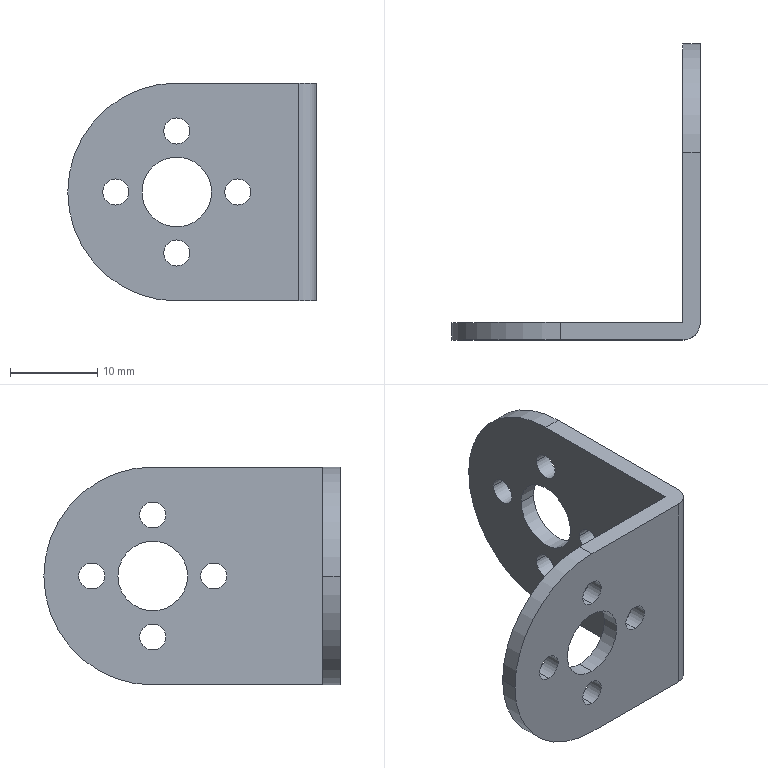Part | SolidWorks | features Fillet 3, ICE 3, Extrusion 1 | 1 solid | 31 faces | box 28.5 x 34 x 25 mm | volume 2421 mm3 | cylinder 25 | plane 6 | commonest cylinder face diameters 3 x16 8 x4 25 x4 4 x1
STEP:
#1=CARTESIAN_POINT('',(-8.75,-15.,14.));
#2=VERTEX_POINT('',#1);
#3=CARTESIAN_POINT('',(-8.75,-15.,11.));
#4=VERTEX_POINT('',#3);
#5=CARTESIAN_POINT('',(-8.75,-15.,12.5));
#6=DIRECTION('',(0.,-1.,0.));
#7=DIRECTION('',(1.,0.,0.));
#8=AXIS2_PLACEMENT_3D('',#5,#6,#7);
#9=CIRCLE('',#8,1.5);
#10=EDGE_CURVE('',#2,#4,#9,.T.);
#11=ORIENTED_EDGE('',*,*,#10,.F.);
#12=CARTESIAN_POINT('',(-8.75,-17.,14.));
#13=VERTEX_POINT('',#12);
#14=CARTESIAN_POINT('',(-8.75,17.,14.));
#15=DIRECTION('',(0.,-1.,0.));
#16=VECTOR('',#15,1000.);
#17=LINE('',#14,#16);
#18=EDGE_CURVE('',#2,#13,#17,.T.);
#19=ORIENTED_EDGE('',*,*,#18,.T.);
#20=CARTESIAN_POINT('',(-8.75,-17.,11.));
#21=VERTEX_POINT('',#20);
#22=CARTESIAN_POINT('',(-8.75,-17.,12.5));
#23=DIRECTION('',(0.,-1.,0.));
#24=DIRECTION('',(0.,0.,-1.));
#25=AXIS2_PLACEMENT_3D('',#22,#23,#24);
#26=CIRCLE('',#25,1.5);
#27=EDGE_CURVE('',#13,#21,#26,.T.);
#28=ORIENTED_EDGE('',*,*,#27,.T.);
#29=CARTESIAN_POINT('',(-8.75,17.,11.));
#30=DIRECTION('',(0.,-1.,0.));
#31=VECTOR('',#30,1000.);
#32=LINE('',#29,#31);
#33=EDGE_CURVE('',#4,#21,#32,.T.);
#34=ORIENTED_EDGE('',*,*,#33,.F.);
#35=EDGE_LOOP('',(#11,#19,#28,#34));
#36=FACE_OUTER_BOUND('',#35,.T.);
#37=CARTESIAN_POINT('',(-8.75,17.,12.5));
#38=DIRECTION('',(0.,-1.,0.));
#39=DIRECTION('',(0.,0.,-1.));
#40=AXIS2_PLACEMENT_3D('',#37,#38,#39);
#41=CYLINDRICAL_SURFACE('',#40,1.5);
#42=ADVANCED_FACE('',(#36),#41,.F.);
#43=CARTESIAN_POINT('',(-1.75,-15.,21.));
#44=VERTEX_POINT('',#43);
#45=CARTESIAN_POINT('',(-1.75,-15.,18.));
#46=VERTEX_POINT('',#45);
#47=CARTESIAN_POINT('',(-1.75,-15.,19.5));
#48=DIRECTION('',(0.,-1.,0.));
#49=DIRECTION('',(1.,0.,0.));
#50=AXIS2_PLACEMENT_3D('',#47,#48,#49);
#51=CIRCLE('',#50,1.5);
#52=EDGE_CURVE('',#44,#46,#51,.T.);
#53=ORIENTED_EDGE('',*,*,#52,.F.);
#54=CARTESIAN_POINT('',(-1.75,-17.,21.));
#55=VERTEX_POINT('',#54);
#56=CARTESIAN_POINT('',(-1.75,17.,21.));
#57=DIRECTION('',(0.,-1.,0.));
#58=VECTOR('',#57,1000.);
#59=LINE('',#56,#58);
#60=EDGE_CURVE('',#44,#55,#59,.T.);
#61=ORIENTED_EDGE('',*,*,#60,.T.);
#62=CARTESIAN_POINT('',(-1.75,-17.,18.));
#63=VERTEX_POINT('',#62);
#64=CARTESIAN_POINT('',(-1.75,-17.,19.5));
#65=DIRECTION('',(0.,-1.,0.));
#66=DIRECTION('',(0.,0.,-1.));
#67=AXIS2_PLACEMENT_3D('',#64,#65,#66);
#68=CIRCLE('',#67,1.5);
#69=EDGE_CURVE('',#55,#63,#68,.T.);
#70=ORIENTED_EDGE('',*,*,#69,.T.);
#71=CARTESIAN_POINT('',(-1.75,17.,18.));
#72=DIRECTION('',(0.,-1.,0.));
#73=VECTOR('',#72,1000.);
#74=LINE('',#71,#73);
#75=EDGE_CURVE('',#46,#63,#74,.T.);
#76=ORIENTED_EDGE('',*,*,#75,.F.);
#77=EDGE_LOOP('',(#53,#61,#70,#76));
#78=FACE_OUTER_BOUND('',#77,.T.);
#79=CARTESIAN_POINT('',(-1.75,17.,19.5));
#80=DIRECTION('',(0.,-1.,0.));
#81=DIRECTION('',(0.,0.,-1.));
#82=AXIS2_PLACEMENT_3D('',#79,#80,#81);
#83=CYLINDRICAL_SURFACE('',#82,1.5);
#84=ADVANCED_FACE('',(#78),#83,.F.);
#85=CARTESIAN_POINT('',(5.25,-15.,14.));
#86=VERTEX_POINT('',#85);
#87=CARTESIAN_POINT('',(5.25,-15.,11.));
#88=VERTEX_POINT('',#87);
#89=CARTESIAN_POINT('',(5.25,-15.,12.5));
#90=DIRECTION('',(0.,-1.,0.));
#91=DIRECTION('',(1.,0.,0.));
#92=AXIS2_PLACEMENT_3D('',#89,#90,#91);
#93=CIRCLE('',#92,1.5);
#94=EDGE_CURVE('',#86,#88,#93,.T.);
#95=ORIENTED_EDGE('',*,*,#94,.F.);
#96=CARTESIAN_POINT('',(5.25,-17.,14.));
#97=VERTEX_POINT('',#96);
#98=CARTESIAN_POINT('',(5.25,17.,14.));
#99=DIRECTION('',(0.,-1.,0.));
#100=VECTOR('',#99,1000.);
#101=LINE('',#98,#100);
#102=EDGE_CURVE('',#86,#97,#101,.T.);
#103=ORIENTED_EDGE('',*,*,#102,.T.);
#104=CARTESIAN_POINT('',(5.25,-17.,11.));
#105=VERTEX_POINT('',#104);
#106=CARTESIAN_POINT('',(5.25,-17.,12.5));
#107=DIRECTION('',(0.,-1.,0.));
#108=DIRECTION('',(0.,0.,-1.));
#109=AXIS2_PLACEMENT_3D('',#106,#107,#108);
#110=CIRCLE('',#109,1.5);
#111=EDGE_CURVE('',#97,#105,#110,.T.);
#112=ORIENTED_EDGE('',*,*,#111,.T.);
#113=CARTESIAN_POINT('',(5.25,17.,11.));
#114=DIRECTION('',(0.,-1.,0.));
#115=VECTOR('',#114,1000.);
#116=LINE('',#113,#115);
#117=EDGE_CURVE('',#88,#105,#116,.T.);
#118=ORIENTED_EDGE('',*,*,#117,.F.);
#119=EDGE_LOOP('',(#95,#103,#112,#118));
#120=FACE_OUTER_BOUND('',#119,.T.);
#121=CARTESIAN_POINT('',(5.25,17.,12.5));
#122=DIRECTION('',(0.,-1.,0.));
#123=DIRECTION('',(0.,0.,-1.));
#124=AXIS2_PLACEMENT_3D('',#121,#122,#123);
#125=CYLINDRICAL_SURFACE('',#124,1.5);
#126=ADVANCED_FACE('',(#120),#125,.F.);
#127=CARTESIAN_POINT('',(-1.75,-15.,7.));
#128=VERTEX_POINT('',#127);
#129=CARTESIAN_POINT('',(-1.75,-15.,4.));
#130=VERTEX_POINT('',#129);
#131=CARTESIAN_POINT('',(-1.75,-15.,5.5));
#132=DIRECTION('',(0.,-1.,0.));
#133=DIRECTION('',(1.,0.,0.));
#134=AXIS2_PLACEMENT_3D('',#131,#132,#133);
#135=CIRCLE('',#134,1.5);
#136=EDGE_CURVE('',#128,#130,#135,.T.);
#137=ORIENTED_EDGE('',*,*,#136,.F.);
#138=CARTESIAN_POINT('',(-1.75,-17.,7.));
#139=VERTEX_POINT('',#138);
#140=CARTESIAN_POINT('',(-1.75,17.,7.));
#141=DIRECTION('',(0.,-1.,0.));
#142=VECTOR('',#141,1000.);
#143=LINE('',#140,#142);
#144=EDGE_CURVE('',#128,#139,#143,.T.);
#145=ORIENTED_EDGE('',*,*,#144,.T.);
#146=CARTESIAN_POINT('',(-1.75,-17.,4.));
#147=VERTEX_POINT('',#146);
#148=CARTESIAN_POINT('',(-1.75,-17.,5.5));
#149=DIRECTION('',(0.,-1.,0.));
#150=DIRECTION('',(0.,0.,-1.));
#151=AXIS2_PLACEMENT_3D('',#148,#149,#150);
#152=CIRCLE('',#151,1.5);
#153=EDGE_CURVE('',#139,#147,#152,.T.);
#154=ORIENTED_EDGE('',*,*,#153,.T.);
#155=CARTESIAN_POINT('',(-1.75,17.,4.));
#156=DIRECTION('',(0.,-1.,0.));
#157=VECTOR('',#156,1000.);
#158=LINE('',#155,#157);
#159=EDGE_CURVE('',#130,#147,#158,.T.);
#160=ORIENTED_EDGE('',*,*,#159,.F.);
#161=EDGE_LOOP('',(#137,#145,#154,#160));
#162=FACE_OUTER_BOUND('',#161,.T.);
#163=CARTESIAN_POINT('',(-1.75,17.,5.5));
#164=DIRECTION('',(0.,-1.,0.));
#165=DIRECTION('',(0.,0.,-1.));
#166=AXIS2_PLACEMENT_3D('',#163,#164,#165);
#167=CYLINDRICAL_SURFACE('',#166,1.5);
#168=ADVANCED_FACE('',(#162),#167,.F.);
#169=CARTESIAN_POINT('',(-1.75,-15.,16.5));
#170=VERTEX_POINT('',#169);
#171=CARTESIAN_POINT('',(-1.75,-15.,8.5));
#172=VERTEX_POINT('',#171);
#173=CARTESIAN_POINT('',(-1.75,-15.,12.5));
#174=DIRECTION('',(0.,-1.,0.));
#175=DIRECTION('',(1.,0.,0.));
#176=AXIS2_PLACEMENT_3D('',#173,#174,#175);
#177=CIRCLE('',#176,4.);
#178=EDGE_CURVE('',#170,#172,#177,.T.);
#179=ORIENTED_EDGE('',*,*,#178,.F.);
#180=CARTESIAN_POINT('',(-1.75,-17.,16.5));
#181=VERTEX_POINT('',#180);
#182=CARTESIAN_POINT('',(-1.75,17.,16.5));
#183=DIRECTION('',(0.,-1.,0.));
#184=VECTOR('',#183,1000.);
#185=LINE('',#182,#184);
#186=EDGE_CURVE('',#170,#181,#185,.T.);
#187=ORIENTED_EDGE('',*,*,#186,.T.);
#188=CARTESIAN_POINT('',(-1.75,-17.,8.5));
#189=VERTEX_POINT('',#188);
#190=CARTESIAN_POINT('',(-1.75,-17.,12.5));
#191=DIRECTION('',(0.,-1.,0.));
#192=DIRECTION('',(0.,0.,-1.));
#193=AXIS2_PLACEMENT_3D('',#190,#191,#192);
#194=CIRCLE('',#193,4.);
#195=EDGE_CURVE('',#181,#189,#194,.T.);
#196=ORIENTED_EDGE('',*,*,#195,.T.);
#197=CARTESIAN_POINT('',(-1.75,17.,8.5));
#198=DIRECTION('',(0.,-1.,0.));
#199=VECTOR('',#198,1000.);
#200=LINE('',#197,#199);
#201=EDGE_CURVE('',#172,#189,#200,.T.);
#202=ORIENTED_EDGE('',*,*,#201,.F.);
#203=EDGE_LOOP('',(#179,#187,#196,#202));
#204=FACE_OUTER_BOUND('',#203,.T.);
#205=CARTESIAN_POINT('',(-1.75,17.,12.5));
#206=DIRECTION('',(0.,-1.,0.));
#207=DIRECTION('',(0.,0.,-1.));
#208=AXIS2_PLACEMENT_3D('',#205,#206,#207);
#209=CYLINDRICAL_SURFACE('',#208,4.);
#210=ADVANCED_FACE('',(#204),#209,.F.);
#211=CARTESIAN_POINT('',(14.25,6.,5.5));
#212=VERTEX_POINT('',#211);
#213=CARTESIAN_POINT('',(14.25,3.,5.5));
#214=VERTEX_POINT('',#213);
#215=CARTESIAN_POINT('',(14.25,4.5,5.5));
#216=DIRECTION('',(-1.,0.,0.));
#217=DIRECTION('',(0.,-1.,0.));
#218=AXIS2_PLACEMENT_3D('',#215,#216,#217);
#219=CIRCLE('',#218,1.5);
#220=EDGE_CURVE('',#212,#214,#219,.T.);
#221=ORIENTED_EDGE('',*,*,#220,.F.);
#222=CARTESIAN_POINT('',(12.25,6.,5.5));
#223=VERTEX_POINT('',#222);
#224=CARTESIAN_POINT('',(14.25,6.,5.5));
#225=DIRECTION('',(-1.,0.,0.));
#226=VECTOR('',#225,1000.);
#227=LINE('',#224,#226);
#228=EDGE_CURVE('',#212,#223,#227,.T.);
#229=ORIENTED_EDGE('',*,*,#228,.T.);
#230=CARTESIAN_POINT('',(12.25,3.,5.5));
#231=VERTEX_POINT('',#230);
#232=CARTESIAN_POINT('',(12.25,4.5,5.5));
#233=DIRECTION('',(-1.,0.,0.));
#234=DIRECTION('',(0.,-1.,0.));
#235=AXIS2_PLACEMENT_3D('',#232,#233,#234);
#236=CIRCLE('',#235,1.5);
#237=EDGE_CURVE('',#223,#231,#236,.T.);
#238=ORIENTED_EDGE('',*,*,#237,.T.);
#239=CARTESIAN_POINT('',(14.25,3.,5.5));
#240=DIRECTION('',(-1.,0.,0.));
#241=VECTOR('',#240,1000.);
#242=LINE('',#239,#241);
#243=EDGE_CURVE('',#214,#231,#242,.T.);
#244=ORIENTED_EDGE('',*,*,#243,.F.);
#245=EDGE_LOOP('',(#221,#229,#238,#244));
#246=FACE_OUTER_BOUND('',#245,.T.);
#247=CARTESIAN_POINT('',(14.25,4.5,5.5));
#248=DIRECTION('',(-1.,0.,0.));
#249=DIRECTION('',(0.,-1.,0.));
#250=AXIS2_PLACEMENT_3D('',#247,#248,#249);
#251=CYLINDRICAL_SURFACE('',#250,1.5);
#252=ADVANCED_FACE('',(#246),#251,.F.);
#253=CARTESIAN_POINT('',(14.25,13.,12.5));
#254=VERTEX_POINT('',#253);
#255=CARTESIAN_POINT('',(14.25,10.,12.5));
#256=VERTEX_POINT('',#255);
#257=CARTESIAN_POINT('',(14.25,11.5,12.5));
#258=DIRECTION('',(-1.,0.,0.));
#259=DIRECTION('',(0.,-1.,0.));
#260=AXIS2_PLACEMENT_3D('',#257,#258,#259);
#261=CIRCLE('',#260,1.5);
#262=EDGE_CURVE('',#254,#256,#261,.T.);
#263=ORIENTED_EDGE('',*,*,#262,.F.);
#264=CARTESIAN_POINT('',(12.25,13.,12.5));
#265=VERTEX_POINT('',#264);
#266=CARTESIAN_POINT('',(14.25,13.,12.5));
#267=DIRECTION('',(-1.,0.,0.));
#268=VECTOR('',#267,1000.);
#269=LINE('',#266,#268);
#270=EDGE_CURVE('',#254,#265,#269,.T.);
#271=ORIENTED_EDGE('',*,*,#270,.T.);
#272=CARTESIAN_POINT('',(12.25,10.,12.5));
#273=VERTEX_POINT('',#272);
#274=CARTESIAN_POINT('',(12.25,11.5,12.5));
#275=DIRECTION('',(-1.,0.,0.));
#276=DIRECTION('',(0.,-1.,0.));
#277=AXIS2_PLACEMENT_3D('',#274,#275,#276);
#278=CIRCLE('',#277,1.5);
#279=EDGE_CURVE('',#265,#273,#278,.T.);
#280=ORIENTED_EDGE('',*,*,#279,.T.);
#281=CARTESIAN_POINT('',(14.25,10.,12.5));
#282=DIRECTION('',(-1.,0.,0.));
#283=VECTOR('',#282,1000.);
#284=LINE('',#281,#283);
#285=EDGE_CURVE('',#256,#273,#284,.T.);
#286=ORIENTED_EDGE('',*,*,#285,.F.);
#287=EDGE_LOOP('',(#263,#271,#280,#286));
#288=FACE_OUTER_BOUND('',#287,.T.);
#289=CARTESIAN_POINT('',(14.25,11.5,12.5));
#290=DIRECTION('',(-1.,0.,0.));
#291=DIRECTION('',(0.,-1.,0.));
#292=AXIS2_PLACEMENT_3D('',#289,#290,#291);
#293=CYLINDRICAL_SURFACE('',#292,1.5);
#294=ADVANCED_FACE('',(#288),#293,.F.);
#295=CARTESIAN_POINT('',(14.25,6.,19.5));
#296=VERTEX_POINT('',#295);
#297=CARTESIAN_POINT('',(14.25,3.,19.5));
#298=VERTEX_POINT('',#297);
#299=CARTESIAN_POINT('',(14.25,4.5,19.5));
#300=DIRECTION('',(-1.,0.,0.));
#301=DIRECTION('',(0.,-1.,0.));
#302=AXIS2_PLACEMENT_3D('',#299,#300,#301);
#303=CIRCLE('',#302,1.5);
#304=EDGE_CURVE('',#296,#298,#303,.T.);
#305=ORIENTED_EDGE('',*,*,#304,.F.);
#306=CARTESIAN_POINT('',(12.25,6.,19.5));
#307=VERTEX_POINT('',#306);
#308=CARTESIAN_POINT('',(14.25,6.,19.5));
#309=DIRECTION('',(-1.,0.,0.));
#310=VECTOR('',#309,1000.);
#311=LINE('',#308,#310);
#312=EDGE_CURVE('',#296,#307,#311,.T.);
#313=ORIENTED_EDGE('',*,*,#312,.T.);
#314=CARTESIAN_POINT('',(12.25,3.,19.5));
#315=VERTEX_POINT('',#314);
#316=CARTESIAN_POINT('',(12.25,4.5,19.5));
#317=DIRECTION('',(-1.,0.,0.));
#318=DIRECTION('',(0.,-1.,0.));
#319=AXIS2_PLACEMENT_3D('',#316,#317,#318);
#320=CIRCLE('',#319,1.5);
#321=EDGE_CURVE('',#307,#315,#320,.T.);
#322=ORIENTED_EDGE('',*,*,#321,.T.);
#323=CARTESIAN_POINT('',(14.25,3.,19.5));
#324=DIRECTION('',(-1.,0.,0.));
#325=VECTOR('',#324,1000.);
#326=LINE('',#323,#325);
#327=EDGE_CURVE('',#298,#315,#326,.T.);
#328=ORIENTED_EDGE('',*,*,#327,.F.);
#329=EDGE_LOOP('',(#305,#313,#322,#328));
#330=FACE_OUTER_BOUND('',#329,.T.);
#331=CARTESIAN_POINT('',(14.25,4.5,19.5));
#332=DIRECTION('',(-1.,0.,0.));
#333=DIRECTION('',(0.,-1.,0.));
#334=AXIS2_PLACEMENT_3D('',#331,#332,#333);
#335=CYLINDRICAL_SURFACE('',#334,1.5);
#336=ADVANCED_FACE('',(#330),#335,.F.);
#337=CARTESIAN_POINT('',(14.25,-1.,12.5));
#338=VERTEX_POINT('',#337);
#339=CARTESIAN_POINT('',(14.25,-4.,12.5));
#340=VERTEX_POINT('',#339);
#341=CARTESIAN_POINT('',(14.25,-2.5,12.5));
#342=DIRECTION('',(-1.,0.,0.));
#343=DIRECTION('',(0.,-1.,0.));
#344=AXIS2_PLACEMENT_3D('',#341,#342,#343);
#345=CIRCLE('',#344,1.5);
#346=EDGE_CURVE('',#338,#340,#345,.T.);
#347=ORIENTED_EDGE('',*,*,#346,.F.);
#348=CARTESIAN_POINT('',(12.25,-1.,12.5));
#349=VERTEX_POINT('',#348);
#350=CARTESIAN_POINT('',(14.25,-1.,12.5));
#351=DIRECTION('',(-1.,0.,0.));
#352=VECTOR('',#351,1000.);
#353=LINE('',#350,#352);
#354=EDGE_CURVE('',#338,#349,#353,.T.);
#355=ORIENTED_EDGE('',*,*,#354,.T.);
#356=CARTESIAN_POINT('',(12.25,-4.,12.5));
#357=VERTEX_POINT('',#356);
#358=CARTESIAN_POINT('',(12.25,-2.5,12.5));
#359=DIRECTION('',(-1.,0.,0.));
#360=DIRECTION('',(0.,-1.,0.));
#361=AXIS2_PLACEMENT_3D('',#358,#359,#360);
#362=CIRCLE('',#361,1.5);
#363=EDGE_CURVE('',#349,#357,#362,.T.);
#364=ORIENTED_EDGE('',*,*,#363,.T.);
#365=CARTESIAN_POINT('',(14.25,-4.,12.5));
#366=DIRECTION('',(-1.,0.,0.));
#367=VECTOR('',#366,1000.);
#368=LINE('',#365,#367);
#369=EDGE_CURVE('',#340,#357,#368,.T.);
#370=ORIENTED_EDGE('',*,*,#369,.F.);
#371=EDGE_LOOP('',(#347,#355,#364,#370));
#372=FACE_OUTER_BOUND('',#371,.T.);
#373=CARTESIAN_POINT('',(14.25,-2.5,12.5));
#374=DIRECTION('',(-1.,0.,0.));
#375=DIRECTION('',(0.,-1.,0.));
#376=AXIS2_PLACEMENT_3D('',#373,#374,#375);
#377=CYLINDRICAL_SURFACE('',#376,1.5);
#378=ADVANCED_FACE('',(#372),#377,.F.);
#379=CARTESIAN_POINT('',(14.25,8.5,12.5));
#380=VERTEX_POINT('',#379);
#381=CARTESIAN_POINT('',(14.25,0.5,12.5));
#382=VERTEX_POINT('',#381);
#383=CARTESIAN_POINT('',(14.25,4.5,12.5));
#384=DIRECTION('',(-1.,0.,0.));
#385=DIRECTION('',(0.,-1.,0.));
#386=AXIS2_PLACEMENT_3D('',#383,#384,#385);
#387=CIRCLE('',#386,4.);
#388=EDGE_CURVE('',#380,#382,#387,.T.);
#389=ORIENTED_EDGE('',*,*,#388,.F.);
#390=CARTESIAN_POINT('',(12.25,8.5,12.5));
#391=VERTEX_POINT('',#390);
#392=CARTESIAN_POINT('',(14.25,8.5,12.5));
#393=DIRECTION('',(-1.,0.,0.));
#394=VECTOR('',#393,1000.);
#395=LINE('',#392,#394);
#396=EDGE_CURVE('',#380,#391,#395,.T.);
#397=ORIENTED_EDGE('',*,*,#396,.T.);
#398=CARTESIAN_POINT('',(12.25,0.5,12.5));
#399=VERTEX_POINT('',#398);
#400=CARTESIAN_POINT('',(12.25,4.5,12.5));
#401=DIRECTION('',(-1.,0.,0.));
#402=DIRECTION('',(0.,-1.,0.));
#403=AXIS2_PLACEMENT_3D('',#400,#401,#402);
#404=CIRCLE('',#403,4.);
#405=EDGE_CURVE('',#391,#399,#404,.T.);
#406=ORIENTED_EDGE('',*,*,#405,.T.);
#407=CARTESIAN_POINT('',(14.25,0.5,12.5));
#408=DIRECTION('',(-1.,0.,0.));
#409=VECTOR('',#408,1000.);
#410=LINE('',#407,#409);
#411=EDGE_CURVE('',#382,#399,#410,.T.);
#412=ORIENTED_EDGE('',*,*,#411,.F.);
#413=EDGE_LOOP('',(#389,#397,#406,#412));
#414=FACE_OUTER_BOUND('',#413,.T.);
#415=CARTESIAN_POINT('',(14.25,4.5,12.5));
#416=DIRECTION('',(-1.,0.,0.));
#417=DIRECTION('',(0.,-1.,0.));
#418=AXIS2_PLACEMENT_3D('',#415,#416,#417);
#419=CYLINDRICAL_SURFACE('',#418,4.);
#420=ADVANCED_FACE('',(#414),#419,.F.);
#421=CARTESIAN_POINT('',(14.25,4.5,5.5));
#422=DIRECTION('',(-1.,0.,0.));
#423=DIRECTION('',(0.,-1.,0.));
#424=AXIS2_PLACEMENT_3D('',#421,#422,#423);
#425=CIRCLE('',#424,1.5);
#426=EDGE_CURVE('',#214,#212,#425,.T.);
#427=ORIENTED_EDGE('',*,*,#426,.T.);
#428=ORIENTED_EDGE('',*,*,#220,.T.);
#429=EDGE_LOOP('',(#427,#428));
#430=FACE_BOUND('',#429,.T.);
#431=CARTESIAN_POINT('',(14.25,11.5,12.5));
#432=DIRECTION('',(-1.,0.,0.));
#433=DIRECTION('',(0.,-1.,0.));
#434=AXIS2_PLACEMENT_3D('',#431,#432,#433);
#435=CIRCLE('',#434,1.5);
#436=EDGE_CURVE('',#256,#254,#435,.T.);
#437=ORIENTED_EDGE('',*,*,#436,.T.);
#438=ORIENTED_EDGE('',*,*,#262,.T.);
#439=EDGE_LOOP('',(#437,#438));
#440=FACE_BOUND('',#439,.T.);
#441=CARTESIAN_POINT('',(14.25,4.5,19.5));
#442=DIRECTION('',(-1.,0.,0.));
#443=DIRECTION('',(0.,-1.,0.));
#444=AXIS2_PLACEMENT_3D('',#441,#442,#443);
#445=CIRCLE('',#444,1.5);
#446=EDGE_CURVE('',#298,#296,#445,.T.);
#447=ORIENTED_EDGE('',*,*,#446,.T.);
#448=ORIENTED_EDGE('',*,*,#304,.T.);
#449=EDGE_LOOP('',(#447,#448));
#450=FACE_BOUND('',#449,.T.);
#451=CARTESIAN_POINT('',(14.25,-2.5,12.5));
#452=DIRECTION('',(-1.,0.,0.));
#453=DIRECTION('',(0.,-1.,0.));
#454=AXIS2_PLACEMENT_3D('',#451,#452,#453);
#455=CIRCLE('',#454,1.5);
#456=EDGE_CURVE('',#340,#338,#455,.T.);
#457=ORIENTED_EDGE('',*,*,#456,.T.);
#458=ORIENTED_EDGE('',*,*,#346,.T.);
#459=EDGE_LOOP('',(#457,#458));
#460=FACE_BOUND('',#459,.T.);
#461=CARTESIAN_POINT('',(14.25,4.5,12.5));
#462=DIRECTION('',(-1.,0.,0.));
#463=DIRECTION('',(0.,-1.,0.));
#464=AXIS2_PLACEMENT_3D('',#461,#462,#463);
#465=CIRCLE('',#464,4.);
#466=EDGE_CURVE('',#382,#380,#465,.T.);
#467=ORIENTED_EDGE('',*,*,#466,.T.);
#468=ORIENTED_EDGE('',*,*,#388,.T.);
#469=EDGE_LOOP('',(#467,#468));
#470=FACE_BOUND('',#469,.T.);
#471=CARTESIAN_POINT('',(14.25,-15.,25.));
#472=VERTEX_POINT('',#471);
#473=CARTESIAN_POINT('',(14.25,4.5,25.));
#474=VERTEX_POINT('',#473);
#475=CARTESIAN_POINT('',(14.25,17.,25.));
#476=DIRECTION('',(0.,1.,0.));
#477=VECTOR('',#476,1000.);
#478=LINE('',#475,#477);
#479=EDGE_CURVE('',#472,#474,#478,.T.);
#480=ORIENTED_EDGE('',*,*,#479,.F.);
#481=CARTESIAN_POINT('',(14.25,-15.,0.));
#482=VERTEX_POINT('',#481);
#483=CARTESIAN_POINT('',(14.25,-15.,25.));
#484=DIRECTION('',(0.,0.,-1.));
#485=VECTOR('',#484,1000.);
#486=LINE('',#483,#485);
#487=EDGE_CURVE('',#472,#482,#486,.T.);
#488=ORIENTED_EDGE('',*,*,#487,.T.);
#489=CARTESIAN_POINT('',(14.25,4.5,0.));
#490=VERTEX_POINT('',#489);
#491=CARTESIAN_POINT('',(14.25,17.,0.));
#492=DIRECTION('',(0.,1.,0.));
#493=VECTOR('',#492,1000.);
#494=LINE('',#491,#493);
#495=EDGE_CURVE('',#482,#490,#494,.T.);
#496=ORIENTED_EDGE('',*,*,#495,.T.);
#497=CARTESIAN_POINT('',(14.25,17.,12.5));
#498=VERTEX_POINT('',#497);
#499=CARTESIAN_POINT('',(14.25,4.5,12.5));
#500=DIRECTION('',(1.,0.,0.));
#501=DIRECTION('',(0.,-1.,0.));
#502=AXIS2_PLACEMENT_3D('',#499,#500,#501);
#503=CIRCLE('',#502,12.5);
#504=EDGE_CURVE('',#490,#498,#503,.T.);
#505=ORIENTED_EDGE('',*,*,#504,.T.);
#506=CARTESIAN_POINT('',(14.25,4.5,12.5));
#507=DIRECTION('',(1.,0.,0.));
#508=DIRECTION('',(0.,-1.,0.));
#509=AXIS2_PLACEMENT_3D('',#506,#507,#508);
#510=CIRCLE('',#509,12.5);
#511=EDGE_CURVE('',#498,#474,#510,.T.);
#512=ORIENTED_EDGE('',*,*,#511,.T.);
#513=EDGE_LOOP('',(#480,#488,#496,#505,#512));
#514=FACE_OUTER_BOUND('',#513,.T.);
#515=CARTESIAN_POINT('',(14.25,17.,25.));
#516=DIRECTION('',(-1.,0.,0.));
#517=DIRECTION('',(0.,-1.,0.));
#518=AXIS2_PLACEMENT_3D('',#515,#516,#517);
#519=PLANE('',#518);
#520=ADVANCED_FACE('',(#430,#440,#450,#460,#470,#514),#519,.F.);
#521=CARTESIAN_POINT('',(-8.75,-17.,12.5));
#522=DIRECTION('',(0.,-1.,0.));
#523=DIRECTION('',(0.,0.,-1.));
#524=AXIS2_PLACEMENT_3D('',#521,#522,#523);
#525=CIRCLE('',#524,1.5);
#526=EDGE_CURVE('',#21,#13,#525,.T.);
#527=ORIENTED_EDGE('',*,*,#526,.F.);
#528=ORIENTED_EDGE('',*,*,#27,.F.);
#529=EDGE_LOOP('',(#527,#528));
#530=FACE_BOUND('',#529,.T.);
#531=CARTESIAN_POINT('',(-1.75,-17.,19.5));
#532=DIRECTION('',(0.,-1.,0.));
#533=DIRECTION('',(0.,0.,-1.));
#534=AXIS2_PLACEMENT_3D('',#531,#532,#533);
#535=CIRCLE('',#534,1.5);
#536=EDGE_CURVE('',#63,#55,#535,.T.);
#537=ORIENTED_EDGE('',*,*,#536,.F.);
#538=ORIENTED_EDGE('',*,*,#69,.F.);
#539=EDGE_LOOP('',(#537,#538));
#540=FACE_BOUND('',#539,.T.);
#541=CARTESIAN_POINT('',(5.25,-17.,12.5));
#542=DIRECTION('',(0.,-1.,0.));
#543=DIRECTION('',(0.,0.,-1.));
#544=AXIS2_PLACEMENT_3D('',#541,#542,#543);
#545=CIRCLE('',#544,1.5);
#546=EDGE_CURVE('',#105,#97,#545,.T.);
#547=ORIENTED_EDGE('',*,*,#546,.F.);
#548=ORIENTED_EDGE('',*,*,#111,.F.);
#549=EDGE_LOOP('',(#547,#548));
#550=FACE_BOUND('',#549,.T.);
#551=CARTESIAN_POINT('',(-1.75,-17.,5.5));
#552=DIRECTION('',(0.,-1.,0.));
#553=DIRECTION('',(0.,0.,-1.));
#554=AXIS2_PLACEMENT_3D('',#551,#552,#553);
#555=CIRCLE('',#554,1.5);
#556=EDGE_CURVE('',#147,#139,#555,.T.);
#557=ORIENTED_EDGE('',*,*,#556,.F.);
#558=ORIENTED_EDGE('',*,*,#153,.F.);
#559=EDGE_LOOP('',(#557,#558));
#560=FACE_BOUND('',#559,.T.);
#561=CARTESIAN_POINT('',(-1.75,-17.,12.5));
#562=DIRECTION('',(0.,-1.,0.));
#563=DIRECTION('',(0.,0.,-1.));
#564=AXIS2_PLACEMENT_3D('',#561,#562,#563);
#565=CIRCLE('',#564,4.);
#566=EDGE_CURVE('',#189,#181,#565,.T.);
#567=ORIENTED_EDGE('',*,*,#566,.F.);
#568=ORIENTED_EDGE('',*,*,#195,.F.);
#569=EDGE_LOOP('',(#567,#568));
#570=FACE_BOUND('',#569,.T.);
#571=CARTESIAN_POINT('',(-1.75,-17.,0.));
#572=VERTEX_POINT('',#571);
#573=CARTESIAN_POINT('',(12.25,-17.,0.));
#574=VERTEX_POINT('',#573);
#575=CARTESIAN_POINT('',(-14.25,-17.,0.));
#576=DIRECTION('',(1.,0.,0.));
#577=VECTOR('',#576,1000.);
#578=LINE('',#575,#577);
#579=EDGE_CURVE('',#572,#574,#578,.T.);
#580=ORIENTED_EDGE('',*,*,#579,.T.);
#581=CARTESIAN_POINT('',(12.25,-17.,25.));
#582=VERTEX_POINT('',#581);
#583=CARTESIAN_POINT('',(12.25,-17.,25.));
#584=DIRECTION('',(0.,0.,1.));
#585=VECTOR('',#584,1000.);
#586=LINE('',#583,#585);
#587=EDGE_CURVE('',#574,#582,#586,.T.);
#588=ORIENTED_EDGE('',*,*,#587,.T.);
#589=CARTESIAN_POINT('',(-1.75,-17.,25.));
#590=VERTEX_POINT('',#589);
#591=CARTESIAN_POINT('',(-14.25,-17.,25.));
#592=DIRECTION('',(1.,0.,0.));
#593=VECTOR('',#592,1000.);
#594=LINE('',#591,#593);
#595=EDGE_CURVE('',#590,#582,#594,.T.);
#596=ORIENTED_EDGE('',*,*,#595,.F.);
#597=CARTESIAN_POINT('',(-14.25,-17.,12.5));
#598=VERTEX_POINT('',#597);
#599=CARTESIAN_POINT('',(-1.75,-17.,12.5));
#600=DIRECTION('',(0.,-1.,0.));
#601=DIRECTION('',(0.,0.,1.));
#602=AXIS2_PLACEMENT_3D('',#599,#600,#601);
#603=CIRCLE('',#602,12.5);
#604=EDGE_CURVE('',#590,#598,#603,.T.);
#605=ORIENTED_EDGE('',*,*,#604,.T.);
#606=CARTESIAN_POINT('',(-1.75,-17.,12.5));
#607=DIRECTION('',(0.,-1.,0.));
#608=DIRECTION('',(0.,0.,1.));
#609=AXIS2_PLACEMENT_3D('',#606,#607,#608);
#610=CIRCLE('',#609,12.5);
#611=EDGE_CURVE('',#598,#572,#610,.T.);
#612=ORIENTED_EDGE('',*,*,#611,.T.);
#613=EDGE_LOOP('',(#580,#588,#596,#605,#612));
#614=FACE_OUTER_BOUND('',#613,.T.);
#615=CARTESIAN_POINT('',(-14.25,-17.,25.));
#616=DIRECTION('',(0.,1.,0.));
#617=DIRECTION('',(0.,0.,1.));
#618=AXIS2_PLACEMENT_3D('',#615,#616,#617);
#619=PLANE('',#618);
#620=ADVANCED_FACE('',(#530,#540,#550,#560,#570,#614),#619,.F.);
#621=ORIENTED_EDGE('',*,*,#595,.T.);
#622=CARTESIAN_POINT('',(12.25,-15.,25.));
#623=DIRECTION('',(0.,0.,1.));
#624=DIRECTION('',(1.,0.,0.));
#625=AXIS2_PLACEMENT_3D('',#622,#623,#624);
#626=CIRCLE('',#625,2.);
#627=EDGE_CURVE('',#582,#472,#626,.T.);
#628=ORIENTED_EDGE('',*,*,#627,.T.);
#629=ORIENTED_EDGE('',*,*,#479,.T.);
#630=CARTESIAN_POINT('',(12.25,4.5,25.));
#631=VERTEX_POINT('',#630);
#632=CARTESIAN_POINT('',(12.25,4.5,25.));
#633=DIRECTION('',(-1.,0.,0.));
#634=VECTOR('',#633,1000.);
#635=LINE('',#632,#634);
#636=EDGE_CURVE('',#474,#631,#635,.T.);
#637=ORIENTED_EDGE('',*,*,#636,.T.);
#638=CARTESIAN_POINT('',(12.25,-15.,25.));
#639=VERTEX_POINT('',#638);
#640=CARTESIAN_POINT('',(12.25,17.,25.));
#641=DIRECTION('',(0.,-1.,0.));
#642=VECTOR('',#641,1000.);
#643=LINE('',#640,#642);
#644=EDGE_CURVE('',#631,#639,#643,.T.);
#645=ORIENTED_EDGE('',*,*,#644,.T.);
#646=CARTESIAN_POINT('',(-1.75,-15.,25.));
#647=VERTEX_POINT('',#646);
#648=CARTESIAN_POINT('',(12.25,-15.,25.));
#649=DIRECTION('',(-1.,0.,0.));
#650=VECTOR('',#649,1000.);
#651=LINE('',#648,#650);
#652=EDGE_CURVE('',#639,#647,#651,.T.);
#653=ORIENTED_EDGE('',*,*,#652,.T.);
#654=CARTESIAN_POINT('',(-1.75,-17.,25.));
#655=DIRECTION('',(0.,-1.,0.));
#656=VECTOR('',#655,1000.);
#657=LINE('',#654,#656);
#658=EDGE_CURVE('',#647,#590,#657,.T.);
#659=ORIENTED_EDGE('',*,*,#658,.T.);
#660=EDGE_LOOP('',(#621,#628,#629,#637,#645,#653,#659));
#661=FACE_OUTER_BOUND('',#660,.T.);
#662=CARTESIAN_POINT('',(0.,0.,25.));
#663=DIRECTION('',(0.,0.,1.));
#664=DIRECTION('',(1.,0.,0.));
#665=AXIS2_PLACEMENT_3D('',#662,#663,#664);
#666=PLANE('',#665);
#667=ADVANCED_FACE('',(#661),#666,.T.);
#668=ORIENTED_EDGE('',*,*,#495,.F.);
#669=CARTESIAN_POINT('',(12.25,-15.,0.));
#670=DIRECTION('',(0.,0.,-1.));
#671=DIRECTION('',(1.,0.,0.));
#672=AXIS2_PLACEMENT_3D('',#669,#670,#671);
#673=CIRCLE('',#672,2.);
#674=EDGE_CURVE('',#482,#574,#673,.T.);
#675=ORIENTED_EDGE('',*,*,#674,.T.);
#676=ORIENTED_EDGE('',*,*,#579,.F.);
#677=CARTESIAN_POINT('',(-1.75,-15.,0.));
#678=VERTEX_POINT('',#677);
#679=CARTESIAN_POINT('',(-1.75,0.,0.));
#680=DIRECTION('',(0.,1.,0.));
#681=VECTOR('',#680,1000.);
#682=LINE('',#679,#681);
#683=EDGE_CURVE('',#572,#678,#682,.T.);
#684=ORIENTED_EDGE('',*,*,#683,.T.);
#685=CARTESIAN_POINT('',(12.25,-15.,0.));
#686=VERTEX_POINT('',#685);
#687=CARTESIAN_POINT('',(12.25,-15.,0.));
#688=DIRECTION('',(-1.,0.,0.));
#689=VECTOR('',#688,1000.);
#690=LINE('',#687,#689);
#691=EDGE_CURVE('',#686,#678,#690,.T.);
#692=ORIENTED_EDGE('',*,*,#691,.F.);
#693=CARTESIAN_POINT('',(12.25,4.5,0.));
#694=VERTEX_POINT('',#693);
#695=CARTESIAN_POINT('',(12.25,17.,0.));
#696=DIRECTION('',(0.,-1.,0.));
#697=VECTOR('',#696,1000.);
#698=LINE('',#695,#697);
#699=EDGE_CURVE('',#694,#686,#698,.T.);
#700=ORIENTED_EDGE('',*,*,#699,.F.);
#701=CARTESIAN_POINT('',(0.,4.5,0.));
#702=DIRECTION('',(1.,0.,0.));
#703=VECTOR('',#702,1000.);
#704=LINE('',#701,#703);
#705=EDGE_CURVE('',#694,#490,#704,.T.);
#706=ORIENTED_EDGE('',*,*,#705,.T.);
#707=EDGE_LOOP('',(#668,#675,#676,#684,#692,#700,#706));
#708=FACE_OUTER_BOUND('',#707,.T.);
#709=CARTESIAN_POINT('',(0.,0.,0.));
#710=DIRECTION('',(0.,0.,1.));
#711=DIRECTION('',(1.,0.,0.));
#712=AXIS2_PLACEMENT_3D('',#709,#710,#711);
#713=PLANE('',#712);
#714=ADVANCED_FACE('',(#708),#713,.F.);
#715=CARTESIAN_POINT('',(12.25,4.5,5.5));
#716=DIRECTION('',(-1.,0.,0.));
#717=DIRECTION('',(0.,-1.,0.));
#718=AXIS2_PLACEMENT_3D('',#715,#716,#717);
#719=CIRCLE('',#718,1.5);
#720=EDGE_CURVE('',#231,#223,#719,.T.);
#721=ORIENTED_EDGE('',*,*,#720,.F.);
#722=ORIENTED_EDGE('',*,*,#237,.F.);
#723=EDGE_LOOP('',(#721,#722));
#724=FACE_BOUND('',#723,.T.);
#725=CARTESIAN_POINT('',(12.25,11.5,12.5));
#726=DIRECTION('',(-1.,0.,0.));
#727=DIRECTION('',(0.,-1.,0.));
#728=AXIS2_PLACEMENT_3D('',#725,#726,#727);
#729=CIRCLE('',#728,1.5);
#730=EDGE_CURVE('',#273,#265,#729,.T.);
#731=ORIENTED_EDGE('',*,*,#730,.F.);
#732=ORIENTED_EDGE('',*,*,#279,.F.);
#733=EDGE_LOOP('',(#731,#732));
#734=FACE_BOUND('',#733,.T.);
#735=CARTESIAN_POINT('',(12.25,4.5,19.5));
#736=DIRECTION('',(-1.,0.,0.));
#737=DIRECTION('',(0.,-1.,0.));
#738=AXIS2_PLACEMENT_3D('',#735,#736,#737);
#739=CIRCLE('',#738,1.5);
#740=EDGE_CURVE('',#315,#307,#739,.T.);
#741=ORIENTED_EDGE('',*,*,#740,.F.);
#742=ORIENTED_EDGE('',*,*,#321,.F.);
#743=EDGE_LOOP('',(#741,#742));
#744=FACE_BOUND('',#743,.T.);
#745=CARTESIAN_POINT('',(12.25,-2.5,12.5));
#746=DIRECTION('',(-1.,0.,0.));
#747=DIRECTION('',(0.,-1.,0.));
#748=AXIS2_PLACEMENT_3D('',#745,#746,#747);
#749=CIRCLE('',#748,1.5);
#750=EDGE_CURVE('',#357,#349,#749,.T.);
#751=ORIENTED_EDGE('',*,*,#750,.F.);
#752=ORIENTED_EDGE('',*,*,#363,.F.);
#753=EDGE_LOOP('',(#751,#752));
#754=FACE_BOUND('',#753,.T.);
#755=CARTESIAN_POINT('',(12.25,4.5,12.5));
#756=DIRECTION('',(-1.,0.,0.));
#757=DIRECTION('',(0.,-1.,0.));
#758=AXIS2_PLACEMENT_3D('',#755,#756,#757);
#759=CIRCLE('',#758,4.);
#760=EDGE_CURVE('',#399,#391,#759,.T.);
#761=ORIENTED_EDGE('',*,*,#760,.F.);
#762=ORIENTED_EDGE('',*,*,#405,.F.);
#763=EDGE_LOOP('',(#761,#762));
#764=FACE_BOUND('',#763,.T.);
#765=ORIENTED_EDGE('',*,*,#644,.F.);
#766=CARTESIAN_POINT('',(12.25,17.,12.5));
#767=VERTEX_POINT('',#766);
#768=CARTESIAN_POINT('',(12.25,4.5,12.5));
#769=DIRECTION('',(-1.,0.,0.));
#770=DIRECTION('',(0.,1.,0.));
#771=AXIS2_PLACEMENT_3D('',#768,#769,#770);
#772=CIRCLE('',#771,12.5);
#773=EDGE_CURVE('',#631,#767,#772,.T.);
#774=ORIENTED_EDGE('',*,*,#773,.T.);
#775=CARTESIAN_POINT('',(12.25,4.5,12.5));
#776=DIRECTION('',(-1.,0.,0.));
#777=DIRECTION('',(0.,1.,0.));
#778=AXIS2_PLACEMENT_3D('',#775,#776,#777);
#779=CIRCLE('',#778,12.5);
#780=EDGE_CURVE('',#767,#694,#779,.T.);
#781=ORIENTED_EDGE('',*,*,#780,.T.);
#782=ORIENTED_EDGE('',*,*,#699,.T.);
#783=CARTESIAN_POINT('',(12.25,-15.,25.));
#784=DIRECTION('',(0.,0.,-1.));
#785=VECTOR('',#784,1000.);
#786=LINE('',#783,#785);
#787=EDGE_CURVE('',#639,#686,#786,.T.);
#788=ORIENTED_EDGE('',*,*,#787,.F.);
#789=EDGE_LOOP('',(#765,#774,#781,#782,#788));
#790=FACE_OUTER_BOUND('',#789,.T.);
#791=CARTESIAN_POINT('',(12.25,17.,25.));
#792=DIRECTION('',(1.,0.,0.));
#793=DIRECTION('',(0.,1.,0.));
#794=AXIS2_PLACEMENT_3D('',#791,#792,#793);
#795=PLANE('',#794);
#796=ADVANCED_FACE('',(#724,#734,#744,#754,#764,#790),#795,.F.);
#797=CARTESIAN_POINT('',(-8.75,-15.,12.5));
#798=DIRECTION('',(0.,-1.,0.));
#799=DIRECTION('',(1.,0.,0.));
#800=AXIS2_PLACEMENT_3D('',#797,#798,#799);
#801=CIRCLE('',#800,1.5);
#802=EDGE_CURVE('',#4,#2,#801,.T.);
#803=ORIENTED_EDGE('',*,*,#802,.T.);
#804=ORIENTED_EDGE('',*,*,#10,.T.);
#805=EDGE_LOOP('',(#803,#804));
#806=FACE_BOUND('',#805,.T.);
#807=CARTESIAN_POINT('',(-1.75,-15.,19.5));
#808=DIRECTION('',(0.,-1.,0.));
#809=DIRECTION('',(1.,0.,0.));
#810=AXIS2_PLACEMENT_3D('',#807,#808,#809);
#811=CIRCLE('',#810,1.5);
#812=EDGE_CURVE('',#46,#44,#811,.T.);
#813=ORIENTED_EDGE('',*,*,#812,.T.);
#814=ORIENTED_EDGE('',*,*,#52,.T.);
#815=EDGE_LOOP('',(#813,#814));
#816=FACE_BOUND('',#815,.T.);
#817=CARTESIAN_POINT('',(5.25,-15.,12.5));
#818=DIRECTION('',(0.,-1.,0.));
#819=DIRECTION('',(1.,0.,0.));
#820=AXIS2_PLACEMENT_3D('',#817,#818,#819);
#821=CIRCLE('',#820,1.5);
#822=EDGE_CURVE('',#88,#86,#821,.T.);
#823=ORIENTED_EDGE('',*,*,#822,.T.);
#824=ORIENTED_EDGE('',*,*,#94,.T.);
#825=EDGE_LOOP('',(#823,#824));
#826=FACE_BOUND('',#825,.T.);
#827=CARTESIAN_POINT('',(-1.75,-15.,5.5));
#828=DIRECTION('',(0.,-1.,0.));
#829=DIRECTION('',(1.,0.,0.));
#830=AXIS2_PLACEMENT_3D('',#827,#828,#829);
#831=CIRCLE('',#830,1.5);
#832=EDGE_CURVE('',#130,#128,#831,.T.);
#833=ORIENTED_EDGE('',*,*,#832,.T.);
#834=ORIENTED_EDGE('',*,*,#136,.T.);
#835=EDGE_LOOP('',(#833,#834));
#836=FACE_BOUND('',#835,.T.);
#837=CARTESIAN_POINT('',(-1.75,-15.,12.5));
#838=DIRECTION('',(0.,-1.,0.));
#839=DIRECTION('',(1.,0.,0.));
#840=AXIS2_PLACEMENT_3D('',#837,#838,#839);
#841=CIRCLE('',#840,4.);
#842=EDGE_CURVE('',#172,#170,#841,.T.);
#843=ORIENTED_EDGE('',*,*,#842,.T.);
#844=ORIENTED_EDGE('',*,*,#178,.T.);
#845=EDGE_LOOP('',(#843,#844));
#846=FACE_BOUND('',#845,.T.);
#847=CARTESIAN_POINT('',(-14.25,-15.,12.5));
#848=VERTEX_POINT('',#847);
#849=CARTESIAN_POINT('',(-1.75,-15.,12.5));
#850=DIRECTION('',(0.,1.,0.));
#851=DIRECTION('',(1.,0.,0.));
#852=AXIS2_PLACEMENT_3D('',#849,#850,#851);
#853=CIRCLE('',#852,12.5);
#854=EDGE_CURVE('',#678,#848,#853,.T.);
#855=ORIENTED_EDGE('',*,*,#854,.T.);
#856=CARTESIAN_POINT('',(-1.75,-15.,12.5));
#857=DIRECTION('',(0.,1.,0.));
#858=DIRECTION('',(1.,0.,0.));
#859=AXIS2_PLACEMENT_3D('',#856,#857,#858);
#860=CIRCLE('',#859,12.5);
#861=EDGE_CURVE('',#848,#647,#860,.T.);
#862=ORIENTED_EDGE('',*,*,#861,.T.);
#863=ORIENTED_EDGE('',*,*,#652,.F.);
#864=ORIENTED_EDGE('',*,*,#787,.T.);
#865=ORIENTED_EDGE('',*,*,#691,.T.);
#866=EDGE_LOOP('',(#855,#862,#863,#864,#865));
#867=FACE_OUTER_BOUND('',#866,.T.);
#868=CARTESIAN_POINT('',(12.25,-15.,25.));
#869=DIRECTION('',(0.,-1.,0.));
#870=DIRECTION('',(1.,0.,0.));
#871=AXIS2_PLACEMENT_3D('',#868,#869,#870);
#872=PLANE('',#871);
#873=ADVANCED_FACE('',(#806,#816,#826,#836,#846,#867),#872,.F.);
#874=ORIENTED_EDGE('',*,*,#396,.F.);
#875=ORIENTED_EDGE('',*,*,#466,.F.);
#876=ORIENTED_EDGE('',*,*,#411,.T.);
#877=ORIENTED_EDGE('',*,*,#760,.T.);
#878=EDGE_LOOP('',(#874,#875,#876,#877));
#879=FACE_OUTER_BOUND('',#878,.T.);
#880=CARTESIAN_POINT('',(14.25,4.5,12.5));
#881=DIRECTION('',(-1.,0.,0.));
#882=DIRECTION('',(0.,-1.,0.));
#883=AXIS2_PLACEMENT_3D('',#880,#881,#882);
#884=CYLINDRICAL_SURFACE('',#883,4.);
#885=ADVANCED_FACE('',(#879),#884,.F.);
#886=ORIENTED_EDGE('',*,*,#354,.F.);
#887=ORIENTED_EDGE('',*,*,#456,.F.);
#888=ORIENTED_EDGE('',*,*,#369,.T.);
#889=ORIENTED_EDGE('',*,*,#750,.T.);
#890=EDGE_LOOP('',(#886,#887,#888,#889));
#891=FACE_OUTER_BOUND('',#890,.T.);
#892=CARTESIAN_POINT('',(14.25,-2.5,12.5));
#893=DIRECTION('',(-1.,0.,0.));
#894=DIRECTION('',(0.,-1.,0.));
#895=AXIS2_PLACEMENT_3D('',#892,#893,#894);
#896=CYLINDRICAL_SURFACE('',#895,1.5);
#897=ADVANCED_FACE('',(#891),#896,.F.);
#898=ORIENTED_EDGE('',*,*,#312,.F.);
#899=ORIENTED_EDGE('',*,*,#446,.F.);
#900=ORIENTED_EDGE('',*,*,#327,.T.);
#901=ORIENTED_EDGE('',*,*,#740,.T.);
#902=EDGE_LOOP('',(#898,#899,#900,#901));
#903=FACE_OUTER_BOUND('',#902,.T.);
#904=CARTESIAN_POINT('',(14.25,4.5,19.5));
#905=DIRECTION('',(-1.,0.,0.));
#906=DIRECTION('',(0.,-1.,0.));
#907=AXIS2_PLACEMENT_3D('',#904,#905,#906);
#908=CYLINDRICAL_SURFACE('',#907,1.5);
#909=ADVANCED_FACE('',(#903),#908,.F.);
#910=ORIENTED_EDGE('',*,*,#270,.F.);
#911=ORIENTED_EDGE('',*,*,#436,.F.);
#912=ORIENTED_EDGE('',*,*,#285,.T.);
#913=ORIENTED_EDGE('',*,*,#730,.T.);
#914=EDGE_LOOP('',(#910,#911,#912,#913));
#915=FACE_OUTER_BOUND('',#914,.T.);
#916=CARTESIAN_POINT('',(14.25,11.5,12.5));
#917=DIRECTION('',(-1.,0.,0.));
#918=DIRECTION('',(0.,-1.,0.));
#919=AXIS2_PLACEMENT_3D('',#916,#917,#918);
#920=CYLINDRICAL_SURFACE('',#919,1.5);
#921=ADVANCED_FACE('',(#915),#920,.F.);
#922=ORIENTED_EDGE('',*,*,#228,.F.);
#923=ORIENTED_EDGE('',*,*,#426,.F.);
#924=ORIENTED_EDGE('',*,*,#243,.T.);
#925=ORIENTED_EDGE('',*,*,#720,.T.);
#926=EDGE_LOOP('',(#922,#923,#924,#925));
#927=FACE_OUTER_BOUND('',#926,.T.);
#928=CARTESIAN_POINT('',(14.25,4.5,5.5));
#929=DIRECTION('',(-1.,0.,0.));
#930=DIRECTION('',(0.,-1.,0.));
#931=AXIS2_PLACEMENT_3D('',#928,#929,#930);
#932=CYLINDRICAL_SURFACE('',#931,1.5);
#933=ADVANCED_FACE('',(#927),#932,.F.);
#934=CARTESIAN_POINT('',(-14.25,17.,12.5));
#935=DIRECTION('',(-1.,0.,0.));
#936=VECTOR('',#935,1000.);
#937=LINE('',#934,#936);
#938=EDGE_CURVE('',#498,#767,#937,.T.);
#939=ORIENTED_EDGE('',*,*,#938,.F.);
#940=ORIENTED_EDGE('',*,*,#504,.F.);
#941=ORIENTED_EDGE('',*,*,#705,.F.);
#942=ORIENTED_EDGE('',*,*,#780,.F.);
#943=EDGE_LOOP('',(#939,#940,#941,#942));
#944=FACE_OUTER_BOUND('',#943,.T.);
#945=CARTESIAN_POINT('',(-14.25,4.5,12.5));
#946=DIRECTION('',(-1.,0.,0.));
#947=DIRECTION('',(0.,0.,1.));
#948=AXIS2_PLACEMENT_3D('',#945,#946,#947);
#949=CYLINDRICAL_SURFACE('',#948,12.5);
#950=ADVANCED_FACE('',(#944),#949,.T.);
#951=ORIENTED_EDGE('',*,*,#511,.F.);
#952=ORIENTED_EDGE('',*,*,#938,.T.);
#953=ORIENTED_EDGE('',*,*,#773,.F.);
#954=ORIENTED_EDGE('',*,*,#636,.F.);
#955=EDGE_LOOP('',(#951,#952,#953,#954));
#956=FACE_OUTER_BOUND('',#955,.T.);
#957=CARTESIAN_POINT('',(0.,4.5,12.5));
#958=DIRECTION('',(1.,0.,0.));
#959=DIRECTION('',(0.,0.,-1.));
#960=AXIS2_PLACEMENT_3D('',#957,#958,#959);
#961=CYLINDRICAL_SURFACE('',#960,12.5);
#962=ADVANCED_FACE('',(#956),#961,.T.);
#963=ORIENTED_EDGE('',*,*,#186,.F.);
#964=ORIENTED_EDGE('',*,*,#842,.F.);
#965=ORIENTED_EDGE('',*,*,#201,.T.);
#966=ORIENTED_EDGE('',*,*,#566,.T.);
#967=EDGE_LOOP('',(#963,#964,#965,#966));
#968=FACE_OUTER_BOUND('',#967,.T.);
#969=CARTESIAN_POINT('',(-1.75,17.,12.5));
#970=DIRECTION('',(0.,-1.,0.));
#971=DIRECTION('',(0.,0.,-1.));
#972=AXIS2_PLACEMENT_3D('',#969,#970,#971);
#973=CYLINDRICAL_SURFACE('',#972,4.);
#974=ADVANCED_FACE('',(#968),#973,.F.);
#975=ORIENTED_EDGE('',*,*,#144,.F.);
#976=ORIENTED_EDGE('',*,*,#832,.F.);
#977=ORIENTED_EDGE('',*,*,#159,.T.);
#978=ORIENTED_EDGE('',*,*,#556,.T.);
#979=EDGE_LOOP('',(#975,#976,#977,#978));
#980=FACE_OUTER_BOUND('',#979,.T.);
#981=CARTESIAN_POINT('',(-1.75,17.,5.5));
#982=DIRECTION('',(0.,-1.,0.));
#983=DIRECTION('',(0.,0.,-1.));
#984=AXIS2_PLACEMENT_3D('',#981,#982,#983);
#985=CYLINDRICAL_SURFACE('',#984,1.5);
#986=ADVANCED_FACE('',(#980),#985,.F.);
#987=ORIENTED_EDGE('',*,*,#102,.F.);
#988=ORIENTED_EDGE('',*,*,#822,.F.);
#989=ORIENTED_EDGE('',*,*,#117,.T.);
#990=ORIENTED_EDGE('',*,*,#546,.T.);
#991=EDGE_LOOP('',(#987,#988,#989,#990));
#992=FACE_OUTER_BOUND('',#991,.T.);
#993=CARTESIAN_POINT('',(5.25,17.,12.5));
#994=DIRECTION('',(0.,-1.,0.));
#995=DIRECTION('',(0.,0.,-1.));
#996=AXIS2_PLACEMENT_3D('',#993,#994,#995);
#997=CYLINDRICAL_SURFACE('',#996,1.5);
#998=ADVANCED_FACE('',(#992),#997,.F.);
#999=ORIENTED_EDGE('',*,*,#60,.F.);
#1000=ORIENTED_EDGE('',*,*,#812,.F.);
#1001=ORIENTED_EDGE('',*,*,#75,.T.);
#1002=ORIENTED_EDGE('',*,*,#536,.T.);
#1003=EDGE_LOOP('',(#999,#1000,#1001,#1002));
#1004=FACE_OUTER_BOUND('',#1003,.T.);
#1005=CARTESIAN_POINT('',(-1.75,17.,19.5));
#1006=DIRECTION('',(0.,-1.,0.));
#1007=DIRECTION('',(0.,0.,-1.));
#1008=AXIS2_PLACEMENT_3D('',#1005,#1006,#1007);
#1009=CYLINDRICAL_SURFACE('',#1008,1.5);
#1010=ADVANCED_FACE('',(#1004),#1009,.F.);
#1011=ORIENTED_EDGE('',*,*,#18,.F.);
#1012=ORIENTED_EDGE('',*,*,#802,.F.);
#1013=ORIENTED_EDGE('',*,*,#33,.T.);
#1014=ORIENTED_EDGE('',*,*,#526,.T.);
#1015=EDGE_LOOP('',(#1011,#1012,#1013,#1014));
#1016=FACE_OUTER_BOUND('',#1015,.T.);
#1017=CARTESIAN_POINT('',(-8.75,17.,12.5));
#1018=DIRECTION('',(0.,-1.,0.));
#1019=DIRECTION('',(0.,0.,-1.));
#1020=AXIS2_PLACEMENT_3D('',#1017,#1018,#1019);
#1021=CYLINDRICAL_SURFACE('',#1020,1.5);
#1022=ADVANCED_FACE('',(#1016),#1021,.F.);
#1023=CARTESIAN_POINT('',(-14.25,17.,12.5));
#1024=DIRECTION('',(0.,-1.,0.));
#1025=VECTOR('',#1024,1000.);
#1026=LINE('',#1023,#1025);
#1027=EDGE_CURVE('',#848,#598,#1026,.T.);
#1028=ORIENTED_EDGE('',*,*,#1027,.F.);
#1029=ORIENTED_EDGE('',*,*,#854,.F.);
#1030=ORIENTED_EDGE('',*,*,#683,.F.);
#1031=ORIENTED_EDGE('',*,*,#611,.F.);
#1032=EDGE_LOOP('',(#1028,#1029,#1030,#1031));
#1033=FACE_OUTER_BOUND('',#1032,.T.);
#1034=CARTESIAN_POINT('',(-1.75,17.,12.5));
#1035=DIRECTION('',(0.,-1.,0.));
#1036=DIRECTION('',(1.,0.,0.));
#1037=AXIS2_PLACEMENT_3D('',#1034,#1035,#1036);
#1038=CYLINDRICAL_SURFACE('',#1037,12.5);
#1039=ADVANCED_FACE('',(#1033),#1038,.T.);
#1040=ORIENTED_EDGE('',*,*,#861,.F.);
#1041=ORIENTED_EDGE('',*,*,#1027,.T.);
#1042=ORIENTED_EDGE('',*,*,#604,.F.);
#1043=ORIENTED_EDGE('',*,*,#658,.F.);
#1044=EDGE_LOOP('',(#1040,#1041,#1042,#1043));
#1045=FACE_OUTER_BOUND('',#1044,.T.);
#1046=CARTESIAN_POINT('',(-1.75,0.,12.5));
#1047=DIRECTION('',(0.,1.,0.));
#1048=DIRECTION('',(-1.,0.,0.));
#1049=AXIS2_PLACEMENT_3D('',#1046,#1047,#1048);
#1050=CYLINDRICAL_SURFACE('',#1049,12.5);
#1051=ADVANCED_FACE('',(#1045),#1050,.T.);
#1052=ORIENTED_EDGE('',*,*,#627,.F.);
#1053=ORIENTED_EDGE('',*,*,#587,.F.);
#1054=ORIENTED_EDGE('',*,*,#674,.F.);
#1055=ORIENTED_EDGE('',*,*,#487,.F.);
#1056=EDGE_LOOP('',(#1052,#1053,#1054,#1055));
#1057=FACE_OUTER_BOUND('',#1056,.T.);
#1058=CARTESIAN_POINT('',(12.25,-15.,25.));
#1059=DIRECTION('',(0.,0.,-1.));
#1060=DIRECTION('',(-1.,0.,0.));
#1061=AXIS2_PLACEMENT_3D('',#1058,#1059,#1060);
#1062=CYLINDRICAL_SURFACE('',#1061,2.);
#1063=ADVANCED_FACE('',(#1057),#1062,.T.);
#1064=CLOSED_SHELL('',(#42,#84,#126,#168,#210,#252,#294,#336,#378,#420,#520,#620,#667,#714,#796,#873,#885,#897,#909,#921,#933,#950,#962,#974,#986,#998,#1010,#1022,#1039,#1051,#1063));
#1065=MANIFOLD_SOLID_BREP('',#1064);
#1066=CARTESIAN_POINT('',(0.,0.,0.));
#1067=DIRECTION('',(0.,0.,1.));
#1068=DIRECTION('',(1.,0.,0.));
#1069=AXIS2_PLACEMENT_3D('',#1066,#1067,#1068);
#1070=(LENGTH_UNIT()NAMED_UNIT(*)SI_UNIT(.MILLI.,.METRE.));
#1071=UNCERTAINTY_MEASURE_WITH_UNIT(LENGTH_MEASURE(0.00001),#1070,'','');
#1072=(NAMED_UNIT(*)PLANE_ANGLE_UNIT()SI_UNIT($,.RADIAN.));
#1073=(NAMED_UNIT(*)SI_UNIT($,.STERADIAN.)SOLID_ANGLE_UNIT());
#1074=(GEOMETRIC_REPRESENTATION_CONTEXT(3)GLOBAL_UNCERTAINTY_ASSIGNED_CONTEXT((#1071))GLOBAL_UNIT_ASSIGNED_CONTEXT((#1070,#1072,#1073))REPRESENTATION_CONTEXT('',''));
#1075=ADVANCED_BREP_SHAPE_REPRESENTATION('',(#1065,#1069),#1074);